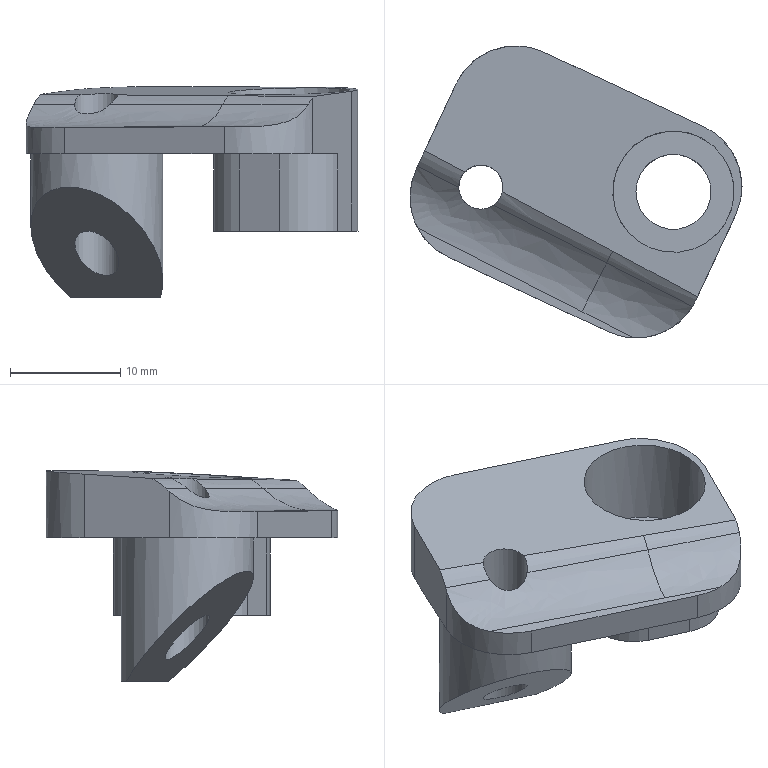Part | STEP file | gslz 2016.10.28-13_id10_x_t | 1 solid | 29 faces | box 30.093 x 26.466 x 19.104 mm | volume 3560 mm3 | plane 12 | cylinder 11 | spline 6 | commonest cylinder face diameters 12 x5 8 x3 4 x1 6.8 x1 11 x1